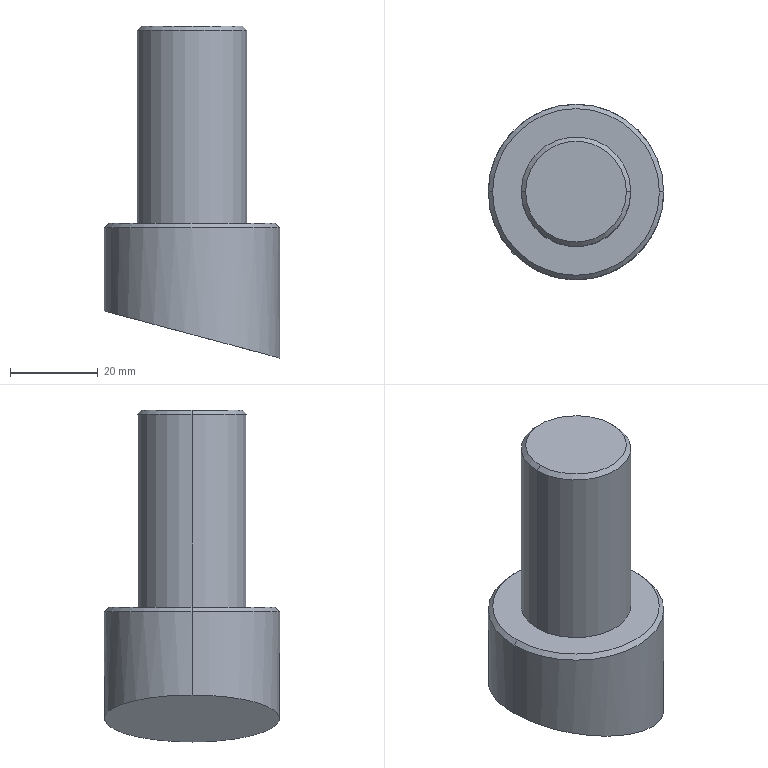Part | SolidWorks | features ICE 2, Chamfer 1, Extrusion 1, RefAxis 1 | 1 solid | 11 faces | box 40 x 40 x 75.72 mm | volume 53860 mm3 | cone 4 | cylinder 4 | plane 3 | commonest cylinder face diameters 25 x2 40 x2
STEP:
#1=CARTESIAN_POINT('',(11.5,0.,75.72));
#2=VERTEX_POINT('',#1);
#3=CARTESIAN_POINT('',(-11.5,0.,75.72));
#4=VERTEX_POINT('',#3);
#5=CARTESIAN_POINT('',(0.,0.,75.72));
#6=DIRECTION('',(0.,0.,1.));
#7=DIRECTION('',(1.,0.,0.));
#8=AXIS2_PLACEMENT_3D('',#5,#6,#7);
#9=CIRCLE('',#8,11.5);
#10=EDGE_CURVE('',#2,#4,#9,.T.);
#11=ORIENTED_EDGE('',*,*,#10,.F.);
#12=CARTESIAN_POINT('',(12.5,0.,74.72));
#13=VERTEX_POINT('',#12);
#14=CARTESIAN_POINT('',(11.5,0.,75.72));
#15=DIRECTION('',(0.7071,0.,-0.7071));
#16=VECTOR('',#15,1000.);
#17=LINE('',#14,#16);
#18=EDGE_CURVE('',#2,#13,#17,.T.);
#19=ORIENTED_EDGE('',*,*,#18,.T.);
#20=CARTESIAN_POINT('',(-12.5,0.,74.72));
#21=VERTEX_POINT('',#20);
#22=CARTESIAN_POINT('',(0.,0.,74.72));
#23=DIRECTION('',(0.,0.,-1.));
#24=DIRECTION('',(1.,0.,0.));
#25=AXIS2_PLACEMENT_3D('',#22,#23,#24);
#26=CIRCLE('',#25,12.5);
#27=EDGE_CURVE('',#21,#13,#26,.T.);
#28=ORIENTED_EDGE('',*,*,#27,.F.);
#29=CARTESIAN_POINT('',(-11.5,0.,75.72));
#30=DIRECTION('',(-0.7071,0.,-0.7071));
#31=VECTOR('',#30,1000.);
#32=LINE('',#29,#31);
#33=EDGE_CURVE('',#4,#21,#32,.T.);
#34=ORIENTED_EDGE('',*,*,#33,.F.);
#35=EDGE_LOOP('',(#11,#19,#28,#34));
#36=FACE_OUTER_BOUND('',#35,.T.);
#37=CARTESIAN_POINT('',(0.,0.,75.72));
#38=DIRECTION('',(0.,0.,-1.));
#39=DIRECTION('',(-1.,0.,0.));
#40=AXIS2_PLACEMENT_3D('',#37,#38,#39);
#41=CONICAL_SURFACE('',#40,11.5,0.7854);
#42=ADVANCED_FACE('',(#36),#41,.T.);
#43=CARTESIAN_POINT('',(19.,0.,30.72));
#44=VERTEX_POINT('',#43);
#45=CARTESIAN_POINT('',(-19.,0.,30.72));
#46=VERTEX_POINT('',#45);
#47=CARTESIAN_POINT('',(0.,0.,30.72));
#48=DIRECTION('',(0.,0.,1.));
#49=DIRECTION('',(1.,0.,0.));
#50=AXIS2_PLACEMENT_3D('',#47,#48,#49);
#51=CIRCLE('',#50,19.);
#52=EDGE_CURVE('',#44,#46,#51,.T.);
#53=ORIENTED_EDGE('',*,*,#52,.F.);
#54=CARTESIAN_POINT('',(20.,0.,29.72));
#55=VERTEX_POINT('',#54);
#56=CARTESIAN_POINT('',(19.,0.,30.72));
#57=DIRECTION('',(0.7071,0.,-0.7071));
#58=VECTOR('',#57,1000.);
#59=LINE('',#56,#58);
#60=EDGE_CURVE('',#44,#55,#59,.T.);
#61=ORIENTED_EDGE('',*,*,#60,.T.);
#62=CARTESIAN_POINT('',(-20.,0.,29.72));
#63=VERTEX_POINT('',#62);
#64=CARTESIAN_POINT('',(0.,0.,29.72));
#65=DIRECTION('',(0.,0.,-1.));
#66=DIRECTION('',(1.,0.,0.));
#67=AXIS2_PLACEMENT_3D('',#64,#65,#66);
#68=CIRCLE('',#67,20.);
#69=EDGE_CURVE('',#63,#55,#68,.T.);
#70=ORIENTED_EDGE('',*,*,#69,.F.);
#71=CARTESIAN_POINT('',(-19.,0.,30.72));
#72=DIRECTION('',(-0.7071,0.,-0.7071));
#73=VECTOR('',#72,1000.);
#74=LINE('',#71,#73);
#75=EDGE_CURVE('',#46,#63,#74,.T.);
#76=ORIENTED_EDGE('',*,*,#75,.F.);
#77=EDGE_LOOP('',(#53,#61,#70,#76));
#78=FACE_OUTER_BOUND('',#77,.T.);
#79=CARTESIAN_POINT('',(0.,0.,30.72));
#80=DIRECTION('',(0.,0.,-1.));
#81=DIRECTION('',(-1.,0.,0.));
#82=AXIS2_PLACEMENT_3D('',#79,#80,#81);
#83=CONICAL_SURFACE('',#82,19.,0.7854);
#84=ADVANCED_FACE('',(#78),#83,.T.);
#85=ORIENTED_EDGE('',*,*,#27,.T.);
#86=CARTESIAN_POINT('',(12.5,0.,30.72));
#87=VERTEX_POINT('',#86);
#88=CARTESIAN_POINT('',(12.5,0.,75.72));
#89=DIRECTION('',(0.,0.,-1.));
#90=VECTOR('',#89,1000.);
#91=LINE('',#88,#90);
#92=EDGE_CURVE('',#13,#87,#91,.T.);
#93=ORIENTED_EDGE('',*,*,#92,.T.);
#94=CARTESIAN_POINT('',(-12.5,0.,30.72));
#95=VERTEX_POINT('',#94);
#96=CARTESIAN_POINT('',(0.,0.,30.72));
#97=DIRECTION('',(0.,0.,1.));
#98=DIRECTION('',(1.,0.,0.));
#99=AXIS2_PLACEMENT_3D('',#96,#97,#98);
#100=CIRCLE('',#99,12.5);
#101=EDGE_CURVE('',#87,#95,#100,.T.);
#102=ORIENTED_EDGE('',*,*,#101,.T.);
#103=CARTESIAN_POINT('',(-12.5,0.,75.72));
#104=DIRECTION('',(0.,0.,-1.));
#105=VECTOR('',#104,1000.);
#106=LINE('',#103,#105);
#107=EDGE_CURVE('',#21,#95,#106,.T.);
#108=ORIENTED_EDGE('',*,*,#107,.F.);
#109=EDGE_LOOP('',(#85,#93,#102,#108));
#110=FACE_OUTER_BOUND('',#109,.T.);
#111=CARTESIAN_POINT('',(0.,0.,75.72));
#112=DIRECTION('',(0.,0.,-1.));
#113=DIRECTION('',(-1.,0.,0.));
#114=AXIS2_PLACEMENT_3D('',#111,#112,#113);
#115=CYLINDRICAL_SURFACE('',#114,12.5);
#116=ADVANCED_FACE('',(#110),#115,.T.);
#117=ORIENTED_EDGE('',*,*,#69,.T.);
#118=CARTESIAN_POINT('',(20.,0.,0.));
#119=VERTEX_POINT('',#118);
#120=CARTESIAN_POINT('',(20.,0.,30.72));
#121=DIRECTION('',(0.,0.,-1.));
#122=VECTOR('',#121,1000.);
#123=LINE('',#120,#122);
#124=EDGE_CURVE('',#55,#119,#123,.T.);
#125=ORIENTED_EDGE('',*,*,#124,.T.);
#126=CARTESIAN_POINT('',(-20.,0.,10.72));
#127=VERTEX_POINT('',#126);
#128=CARTESIAN_POINT('',(20.,0.,0.));
#129=CARTESIAN_POINT('',(20.,40.,0.));
#130=CARTESIAN_POINT('',(-20.,40.,10.72));
#131=CARTESIAN_POINT('',(-20.,0.,10.72));
#132=(BOUNDED_CURVE()B_SPLINE_CURVE(3,(#128,#129,#130,#131),.UNSPECIFIED.,.F.,.T.)B_SPLINE_CURVE_WITH_KNOTS((4,4),(0.,3.142),.UNSPECIFIED.)CURVE()GEOMETRIC_REPRESENTATION_ITEM()RATIONAL_B_SPLINE_CURVE((1.,0.3333,0.3333,1.))REPRESENTATION_ITEM(''));
#133=EDGE_CURVE('',#119,#127,#132,.T.);
#134=ORIENTED_EDGE('',*,*,#133,.T.);
#135=CARTESIAN_POINT('',(-20.,0.,30.72));
#136=DIRECTION('',(0.,0.,-1.));
#137=VECTOR('',#136,1000.);
#138=LINE('',#135,#137);
#139=EDGE_CURVE('',#63,#127,#138,.T.);
#140=ORIENTED_EDGE('',*,*,#139,.F.);
#141=EDGE_LOOP('',(#117,#125,#134,#140));
#142=FACE_OUTER_BOUND('',#141,.T.);
#143=CARTESIAN_POINT('',(0.,0.,30.72));
#144=DIRECTION('',(0.,0.,-1.));
#145=DIRECTION('',(-1.,0.,0.));
#146=AXIS2_PLACEMENT_3D('',#143,#144,#145);
#147=CYLINDRICAL_SURFACE('',#146,20.);
#148=ADVANCED_FACE('',(#142),#147,.T.);
#149=ORIENTED_EDGE('',*,*,#124,.F.);
#150=CARTESIAN_POINT('',(0.,0.,29.72));
#151=DIRECTION('',(0.,0.,-1.));
#152=DIRECTION('',(1.,0.,0.));
#153=AXIS2_PLACEMENT_3D('',#150,#151,#152);
#154=CIRCLE('',#153,20.);
#155=EDGE_CURVE('',#55,#63,#154,.T.);
#156=ORIENTED_EDGE('',*,*,#155,.T.);
#157=ORIENTED_EDGE('',*,*,#139,.T.);
#158=CARTESIAN_POINT('',(-20.,0.,10.72));
#159=CARTESIAN_POINT('',(-20.,-40.,10.72));
#160=CARTESIAN_POINT('',(20.,-40.,0.));
#161=CARTESIAN_POINT('',(20.,0.,0.));
#162=(BOUNDED_CURVE()B_SPLINE_CURVE(3,(#158,#159,#160,#161),.UNSPECIFIED.,.F.,.F.)B_SPLINE_CURVE_WITH_KNOTS((4,4),(3.142,6.283),.UNSPECIFIED.)CURVE()GEOMETRIC_REPRESENTATION_ITEM()RATIONAL_B_SPLINE_CURVE((1.,0.3333,0.3333,1.))REPRESENTATION_ITEM(''));
#163=EDGE_CURVE('',#127,#119,#162,.T.);
#164=ORIENTED_EDGE('',*,*,#163,.T.);
#165=EDGE_LOOP('',(#149,#156,#157,#164));
#166=FACE_OUTER_BOUND('',#165,.T.);
#167=CARTESIAN_POINT('',(0.,0.,30.72));
#168=DIRECTION('',(0.,0.,-1.));
#169=DIRECTION('',(-1.,0.,0.));
#170=AXIS2_PLACEMENT_3D('',#167,#168,#169);
#171=CYLINDRICAL_SURFACE('',#170,20.);
#172=ADVANCED_FACE('',(#166),#171,.T.);
#173=CARTESIAN_POINT('',(0.,0.,30.72));
#174=DIRECTION('',(0.,0.,1.));
#175=DIRECTION('',(1.,0.,0.));
#176=AXIS2_PLACEMENT_3D('',#173,#174,#175);
#177=CIRCLE('',#176,19.);
#178=EDGE_CURVE('',#46,#44,#177,.T.);
#179=ORIENTED_EDGE('',*,*,#178,.T.);
#180=ORIENTED_EDGE('',*,*,#52,.T.);
#181=EDGE_LOOP('',(#179,#180));
#182=FACE_OUTER_BOUND('',#181,.T.);
#183=CARTESIAN_POINT('',(0.,0.,30.72));
#184=DIRECTION('',(0.,0.,1.));
#185=DIRECTION('',(1.,0.,0.));
#186=AXIS2_PLACEMENT_3D('',#183,#184,#185);
#187=CIRCLE('',#186,12.5);
#188=EDGE_CURVE('',#95,#87,#187,.T.);
#189=ORIENTED_EDGE('',*,*,#188,.F.);
#190=ORIENTED_EDGE('',*,*,#101,.F.);
#191=EDGE_LOOP('',(#189,#190));
#192=FACE_BOUND('',#191,.T.);
#193=CARTESIAN_POINT('',(0.,0.,30.72));
#194=DIRECTION('',(0.,0.,1.));
#195=DIRECTION('',(1.,0.,0.));
#196=AXIS2_PLACEMENT_3D('',#193,#194,#195);
#197=PLANE('',#196);
#198=ADVANCED_FACE('',(#182,#192),#197,.T.);
#199=ORIENTED_EDGE('',*,*,#92,.F.);
#200=CARTESIAN_POINT('',(0.,0.,74.72));
#201=DIRECTION('',(0.,0.,-1.));
#202=DIRECTION('',(1.,0.,0.));
#203=AXIS2_PLACEMENT_3D('',#200,#201,#202);
#204=CIRCLE('',#203,12.5);
#205=EDGE_CURVE('',#13,#21,#204,.T.);
#206=ORIENTED_EDGE('',*,*,#205,.T.);
#207=ORIENTED_EDGE('',*,*,#107,.T.);
#208=ORIENTED_EDGE('',*,*,#188,.T.);
#209=EDGE_LOOP('',(#199,#206,#207,#208));
#210=FACE_OUTER_BOUND('',#209,.T.);
#211=CARTESIAN_POINT('',(0.,0.,75.72));
#212=DIRECTION('',(0.,0.,-1.));
#213=DIRECTION('',(-1.,0.,0.));
#214=AXIS2_PLACEMENT_3D('',#211,#212,#213);
#215=CYLINDRICAL_SURFACE('',#214,12.5);
#216=ADVANCED_FACE('',(#210),#215,.T.);
#217=CARTESIAN_POINT('',(0.,0.,75.72));
#218=DIRECTION('',(0.,0.,1.));
#219=DIRECTION('',(1.,0.,0.));
#220=AXIS2_PLACEMENT_3D('',#217,#218,#219);
#221=CIRCLE('',#220,11.5);
#222=EDGE_CURVE('',#4,#2,#221,.T.);
#223=ORIENTED_EDGE('',*,*,#222,.T.);
#224=ORIENTED_EDGE('',*,*,#10,.T.);
#225=EDGE_LOOP('',(#223,#224));
#226=FACE_OUTER_BOUND('',#225,.T.);
#227=CARTESIAN_POINT('',(0.,0.,75.72));
#228=DIRECTION('',(0.,0.,1.));
#229=DIRECTION('',(1.,0.,0.));
#230=AXIS2_PLACEMENT_3D('',#227,#228,#229);
#231=PLANE('',#230);
#232=ADVANCED_FACE('',(#226),#231,.T.);
#233=ORIENTED_EDGE('',*,*,#163,.F.);
#234=ORIENTED_EDGE('',*,*,#133,.F.);
#235=EDGE_LOOP('',(#233,#234));
#236=FACE_OUTER_BOUND('',#235,.T.);
#237=CARTESIAN_POINT('',(20.,-25.,0.));
#238=DIRECTION('',(0.2589,0.,0.9659));
#239=DIRECTION('',(0.9659,0.,-0.2589));
#240=AXIS2_PLACEMENT_3D('',#237,#238,#239);
#241=PLANE('',#240);
#242=ADVANCED_FACE('',(#236),#241,.F.);
#243=ORIENTED_EDGE('',*,*,#60,.F.);
#244=ORIENTED_EDGE('',*,*,#178,.F.);
#245=ORIENTED_EDGE('',*,*,#75,.T.);
#246=ORIENTED_EDGE('',*,*,#155,.F.);
#247=EDGE_LOOP('',(#243,#244,#245,#246));
#248=FACE_OUTER_BOUND('',#247,.T.);
#249=CARTESIAN_POINT('',(0.,0.,30.72));
#250=DIRECTION('',(0.,0.,-1.));
#251=DIRECTION('',(-1.,0.,0.));
#252=AXIS2_PLACEMENT_3D('',#249,#250,#251);
#253=CONICAL_SURFACE('',#252,19.,0.7854);
#254=ADVANCED_FACE('',(#248),#253,.T.);
#255=ORIENTED_EDGE('',*,*,#18,.F.);
#256=ORIENTED_EDGE('',*,*,#222,.F.);
#257=ORIENTED_EDGE('',*,*,#33,.T.);
#258=ORIENTED_EDGE('',*,*,#205,.F.);
#259=EDGE_LOOP('',(#255,#256,#257,#258));
#260=FACE_OUTER_BOUND('',#259,.T.);
#261=CARTESIAN_POINT('',(0.,0.,75.72));
#262=DIRECTION('',(0.,0.,-1.));
#263=DIRECTION('',(-1.,0.,0.));
#264=AXIS2_PLACEMENT_3D('',#261,#262,#263);
#265=CONICAL_SURFACE('',#264,11.5,0.7854);
#266=ADVANCED_FACE('',(#260),#265,.T.);
#267=CLOSED_SHELL('',(#42,#84,#116,#148,#172,#198,#216,#232,#242,#254,#266));
#268=MANIFOLD_SOLID_BREP('',#267);
#269=CARTESIAN_POINT('',(0.,0.,0.));
#270=DIRECTION('',(0.,0.,1.));
#271=DIRECTION('',(1.,0.,0.));
#272=AXIS2_PLACEMENT_3D('',#269,#270,#271);
#273=(LENGTH_UNIT()NAMED_UNIT(*)SI_UNIT(.MILLI.,.METRE.));
#274=UNCERTAINTY_MEASURE_WITH_UNIT(LENGTH_MEASURE(0.00001),#273,'','');
#275=(NAMED_UNIT(*)PLANE_ANGLE_UNIT()SI_UNIT($,.RADIAN.));
#276=(NAMED_UNIT(*)SI_UNIT($,.STERADIAN.)SOLID_ANGLE_UNIT());
#277=(GEOMETRIC_REPRESENTATION_CONTEXT(3)GLOBAL_UNCERTAINTY_ASSIGNED_CONTEXT((#274))GLOBAL_UNIT_ASSIGNED_CONTEXT((#273,#275,#276))REPRESENTATION_CONTEXT('',''));
#278=ADVANCED_BREP_SHAPE_REPRESENTATION('',(#268,#272),#277);